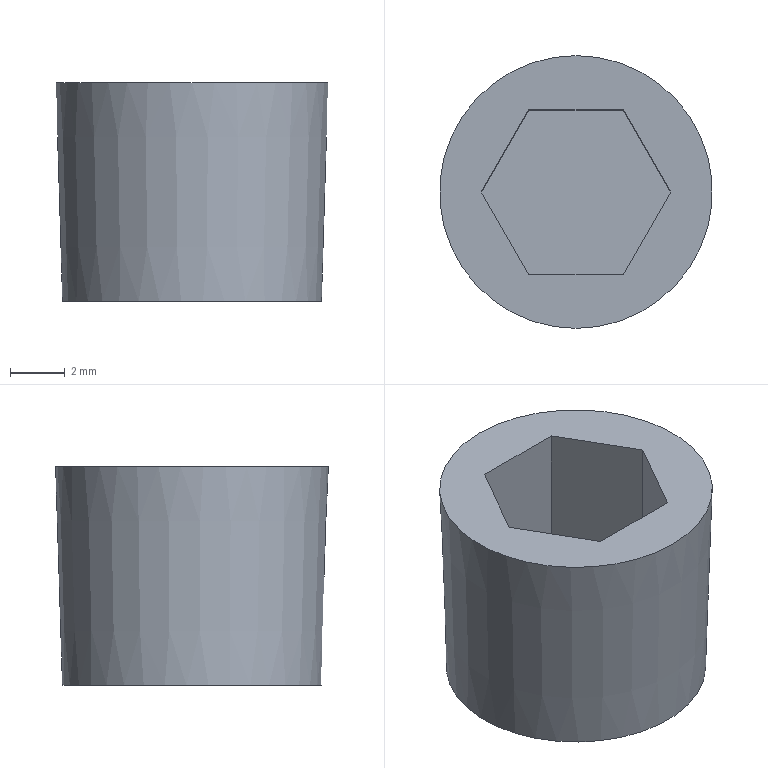Part | STEP file | Cap | 1 solid | 10 faces | volume 438.849 mm3 | plane 9 | cone 1